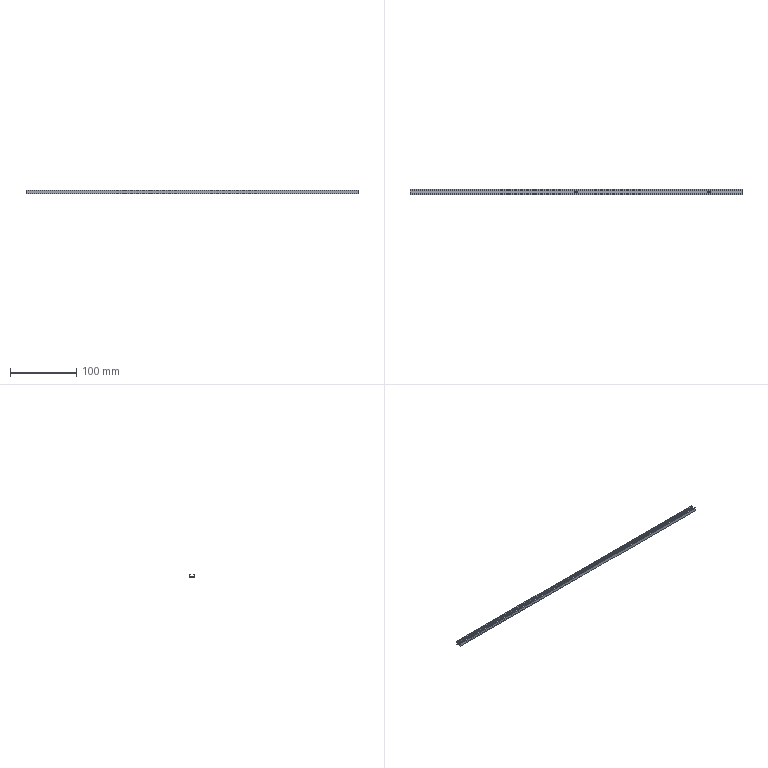Part | STEP file | ASND-0110-KK6010P-600A1-F1CS1-8TCTF01 | 1 solid | 28 faces | box 500 x 8 x 5 mm | volume 9828 mm3 | plane 20 | cylinder 4 | cone 4 | commonest cylinder face diameters 3.12 x4